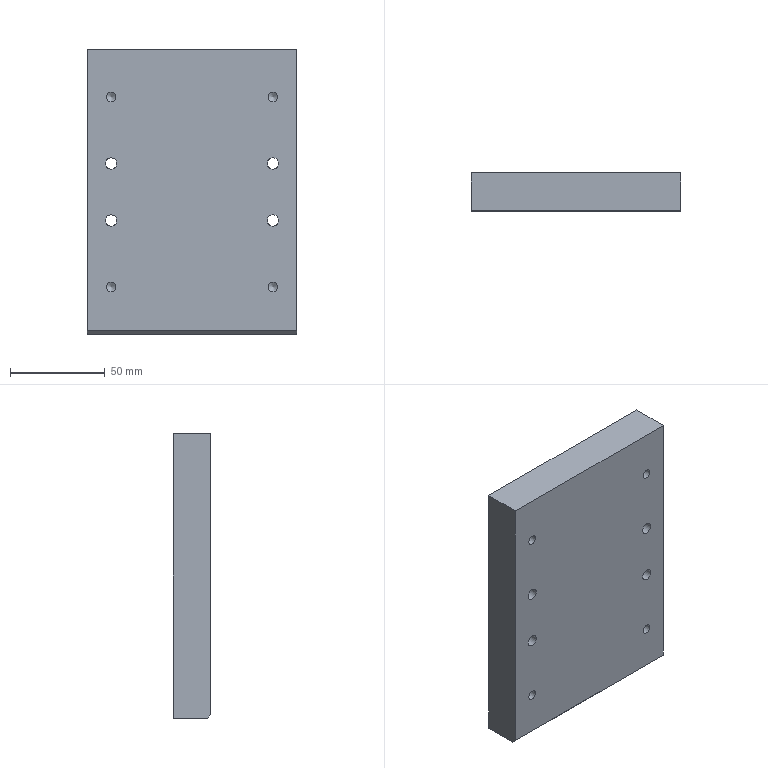Part | NX | features BREP 1 | 1 solid | 23 faces | box 110.2 x 20 x 150 mm | volume 326712 mm3 | plane 11 | cylinder 8 | cone 4 | commonest cylinder face diameters 5 x4 6 x4
STEP:
#1=CARTESIAN_POINT('',(97.7,20.,57.));
#2=VERTEX_POINT('',#1);
#3=CARTESIAN_POINT('',(97.7,20.,60.));
#4=DIRECTION('',(0.,1.,0.));
#5=DIRECTION('',(0.,0.,-1.));
#6=AXIS2_PLACEMENT_3D('',#3,#4,#5);
#7=CIRCLE('',#6,3.);
#8=EDGE_CURVE('',#2,#2,#7,.T.);
#9=ORIENTED_EDGE('',*,*,#8,.F.);
#10=EDGE_LOOP('',(#9));
#11=FACE_BOUND('',#10,.T.);
#12=CARTESIAN_POINT('',(97.7,20.,87.));
#13=VERTEX_POINT('',#12);
#14=CARTESIAN_POINT('',(97.7,20.,90.));
#15=DIRECTION('',(0.,1.,0.));
#16=DIRECTION('',(0.,0.,-1.));
#17=AXIS2_PLACEMENT_3D('',#14,#15,#16);
#18=CIRCLE('',#17,3.);
#19=EDGE_CURVE('',#13,#13,#18,.T.);
#20=ORIENTED_EDGE('',*,*,#19,.F.);
#21=EDGE_LOOP('',(#20));
#22=FACE_BOUND('',#21,.T.);
#23=CARTESIAN_POINT('',(12.5,20.,57.));
#24=VERTEX_POINT('',#23);
#25=CARTESIAN_POINT('',(12.5,20.,60.));
#26=DIRECTION('',(0.,1.,0.));
#27=DIRECTION('',(0.,0.,-1.));
#28=AXIS2_PLACEMENT_3D('',#25,#26,#27);
#29=CIRCLE('',#28,3.);
#30=EDGE_CURVE('',#24,#24,#29,.T.);
#31=ORIENTED_EDGE('',*,*,#30,.F.);
#32=EDGE_LOOP('',(#31));
#33=FACE_BOUND('',#32,.T.);
#34=CARTESIAN_POINT('',(12.5,20.,87.));
#35=VERTEX_POINT('',#34);
#36=CARTESIAN_POINT('',(12.5,20.,90.));
#37=DIRECTION('',(0.,1.,0.));
#38=DIRECTION('',(0.,0.,-1.));
#39=AXIS2_PLACEMENT_3D('',#36,#37,#38);
#40=CIRCLE('',#39,3.);
#41=EDGE_CURVE('',#35,#35,#40,.T.);
#42=ORIENTED_EDGE('',*,*,#41,.F.);
#43=EDGE_LOOP('',(#42));
#44=FACE_BOUND('',#43,.T.);
#45=CARTESIAN_POINT('',(0.,20.,0.));
#46=VERTEX_POINT('',#45);
#47=CARTESIAN_POINT('',(110.2,20.,0.));
#48=VERTEX_POINT('',#47);
#49=CARTESIAN_POINT('',(0.,20.,0.));
#50=DIRECTION('',(1.,0.,0.));
#51=VECTOR('',#50,1000.);
#52=LINE('',#49,#51);
#53=EDGE_CURVE('',#46,#48,#52,.T.);
#54=ORIENTED_EDGE('',*,*,#53,.F.);
#55=CARTESIAN_POINT('',(0.,20.,150.));
#56=VERTEX_POINT('',#55);
#57=CARTESIAN_POINT('',(0.,20.,150.));
#58=DIRECTION('',(0.,0.,-1.));
#59=VECTOR('',#58,1000.);
#60=LINE('',#57,#59);
#61=EDGE_CURVE('',#56,#46,#60,.T.);
#62=ORIENTED_EDGE('',*,*,#61,.F.);
#63=CARTESIAN_POINT('',(110.2,20.,150.));
#64=VERTEX_POINT('',#63);
#65=CARTESIAN_POINT('',(0.,20.,150.));
#66=DIRECTION('',(1.,0.,0.));
#67=VECTOR('',#66,1000.);
#68=LINE('',#65,#67);
#69=EDGE_CURVE('',#56,#64,#68,.T.);
#70=ORIENTED_EDGE('',*,*,#69,.T.);
#71=CARTESIAN_POINT('',(110.2,20.,150.));
#72=DIRECTION('',(0.,0.,-1.));
#73=VECTOR('',#72,1000.);
#74=LINE('',#71,#73);
#75=EDGE_CURVE('',#64,#48,#74,.T.);
#76=ORIENTED_EDGE('',*,*,#75,.T.);
#77=EDGE_LOOP('',(#54,#62,#70,#76));
#78=FACE_BOUND('',#77,.T.);
#79=CARTESIAN_POINT('',(0.,20.,150.));
#80=DIRECTION('',(0.,1.,0.));
#81=DIRECTION('',(1.,0.,0.));
#82=AXIS2_PLACEMENT_3D('',#79,#80,#81);
#83=PLANE('',#82);
#84=ADVANCED_FACE('',(#11,#22,#33,#44,#78),#83,.T.);
#85=CARTESIAN_POINT('',(110.2,0.,150.));
#86=VERTEX_POINT('',#85);
#87=CARTESIAN_POINT('',(110.2,0.,2.));
#88=VERTEX_POINT('',#87);
#89=CARTESIAN_POINT('',(110.2,0.,150.));
#90=DIRECTION('',(0.,0.,-1.));
#91=VECTOR('',#90,1000.);
#92=LINE('',#89,#91);
#93=EDGE_CURVE('',#86,#88,#92,.T.);
#94=ORIENTED_EDGE('',*,*,#93,.T.);
#95=CARTESIAN_POINT('',(110.2,2.,0.));
#96=VERTEX_POINT('',#95);
#97=CARTESIAN_POINT('',(110.2,-64.,66.));
#98=DIRECTION('',(0.,0.7071,-0.7071));
#99=VECTOR('',#98,1000.);
#100=LINE('',#97,#99);
#101=EDGE_CURVE('',#88,#96,#100,.T.);
#102=ORIENTED_EDGE('',*,*,#101,.T.);
#103=CARTESIAN_POINT('',(110.2,20.,0.));
#104=DIRECTION('',(0.,-1.,0.));
#105=VECTOR('',#104,1000.);
#106=LINE('',#103,#105);
#107=EDGE_CURVE('',#48,#96,#106,.T.);
#108=ORIENTED_EDGE('',*,*,#107,.F.);
#109=ORIENTED_EDGE('',*,*,#75,.F.);
#110=CARTESIAN_POINT('',(110.2,20.,150.));
#111=DIRECTION('',(0.,-1.,0.));
#112=VECTOR('',#111,1000.);
#113=LINE('',#110,#112);
#114=EDGE_CURVE('',#64,#86,#113,.T.);
#115=ORIENTED_EDGE('',*,*,#114,.T.);
#116=EDGE_LOOP('',(#94,#102,#108,#109,#115));
#117=FACE_BOUND('',#116,.T.);
#118=CARTESIAN_POINT('',(110.2,20.,150.));
#119=DIRECTION('',(1.,0.,0.));
#120=DIRECTION('',(0.,0.,1.));
#121=AXIS2_PLACEMENT_3D('',#118,#119,#120);
#122=PLANE('',#121);
#123=ADVANCED_FACE('',(#117),#122,.T.);
#124=CARTESIAN_POINT('',(100.7,0.,60.));
#125=VERTEX_POINT('',#124);
#126=CARTESIAN_POINT('',(97.7,0.,60.));
#127=DIRECTION('',(0.,-1.,0.));
#128=DIRECTION('',(1.,0.,0.));
#129=AXIS2_PLACEMENT_3D('',#126,#127,#128);
#130=CIRCLE('',#129,3.);
#131=EDGE_CURVE('',#125,#125,#130,.T.);
#132=ORIENTED_EDGE('',*,*,#131,.F.);
#133=EDGE_LOOP('',(#132));
#134=FACE_BOUND('',#133,.T.);
#135=CARTESIAN_POINT('',(100.7,0.,90.));
#136=VERTEX_POINT('',#135);
#137=CARTESIAN_POINT('',(97.7,0.,90.));
#138=DIRECTION('',(0.,-1.,0.));
#139=DIRECTION('',(1.,0.,0.));
#140=AXIS2_PLACEMENT_3D('',#137,#138,#139);
#141=CIRCLE('',#140,3.);
#142=EDGE_CURVE('',#136,#136,#141,.T.);
#143=ORIENTED_EDGE('',*,*,#142,.F.);
#144=EDGE_LOOP('',(#143));
#145=FACE_BOUND('',#144,.T.);
#146=CARTESIAN_POINT('',(15.5,0.,60.));
#147=VERTEX_POINT('',#146);
#148=CARTESIAN_POINT('',(12.5,0.,60.));
#149=DIRECTION('',(0.,-1.,0.));
#150=DIRECTION('',(1.,0.,0.));
#151=AXIS2_PLACEMENT_3D('',#148,#149,#150);
#152=CIRCLE('',#151,3.);
#153=EDGE_CURVE('',#147,#147,#152,.T.);
#154=ORIENTED_EDGE('',*,*,#153,.F.);
#155=EDGE_LOOP('',(#154));
#156=FACE_BOUND('',#155,.T.);
#157=CARTESIAN_POINT('',(15.5,0.,90.));
#158=VERTEX_POINT('',#157);
#159=CARTESIAN_POINT('',(12.5,0.,90.));
#160=DIRECTION('',(0.,-1.,0.));
#161=DIRECTION('',(1.,0.,0.));
#162=AXIS2_PLACEMENT_3D('',#159,#160,#161);
#163=CIRCLE('',#162,3.);
#164=EDGE_CURVE('',#158,#158,#163,.T.);
#165=ORIENTED_EDGE('',*,*,#164,.F.);
#166=EDGE_LOOP('',(#165));
#167=FACE_BOUND('',#166,.T.);
#168=CARTESIAN_POINT('',(0.,0.,150.));
#169=VERTEX_POINT('',#168);
#170=CARTESIAN_POINT('',(0.,0.,2.));
#171=VERTEX_POINT('',#170);
#172=CARTESIAN_POINT('',(0.,0.,150.));
#173=DIRECTION('',(0.,0.,-1.));
#174=VECTOR('',#173,1000.);
#175=LINE('',#172,#174);
#176=EDGE_CURVE('',#169,#171,#175,.T.);
#177=ORIENTED_EDGE('',*,*,#176,.T.);
#178=CARTESIAN_POINT('',(110.2,0.,2.));
#179=DIRECTION('',(1.,0.,0.));
#180=VECTOR('',#179,1000.);
#181=LINE('',#178,#180);
#182=EDGE_CURVE('',#171,#88,#181,.T.);
#183=ORIENTED_EDGE('',*,*,#182,.T.);
#184=ORIENTED_EDGE('',*,*,#93,.F.);
#185=CARTESIAN_POINT('',(110.2,0.,150.));
#186=DIRECTION('',(-1.,0.,0.));
#187=VECTOR('',#186,1000.);
#188=LINE('',#185,#187);
#189=EDGE_CURVE('',#86,#169,#188,.T.);
#190=ORIENTED_EDGE('',*,*,#189,.T.);
#191=EDGE_LOOP('',(#177,#183,#184,#190));
#192=FACE_BOUND('',#191,.T.);
#193=CARTESIAN_POINT('',(12.5,0.,122.5));
#194=VERTEX_POINT('',#193);
#195=CARTESIAN_POINT('',(12.5,0.,125.));
#196=DIRECTION('',(0.,-1.,0.));
#197=DIRECTION('',(0.,0.,-1.));
#198=AXIS2_PLACEMENT_3D('',#195,#196,#197);
#199=CIRCLE('',#198,2.5);
#200=EDGE_CURVE('',#194,#194,#199,.T.);
#201=ORIENTED_EDGE('',*,*,#200,.F.);
#202=EDGE_LOOP('',(#201));
#203=FACE_BOUND('',#202,.T.);
#204=CARTESIAN_POINT('',(12.5,0.,22.5));
#205=VERTEX_POINT('',#204);
#206=CARTESIAN_POINT('',(12.5,0.,25.));
#207=DIRECTION('',(0.,-1.,0.));
#208=DIRECTION('',(0.,0.,-1.));
#209=AXIS2_PLACEMENT_3D('',#206,#207,#208);
#210=CIRCLE('',#209,2.5);
#211=EDGE_CURVE('',#205,#205,#210,.T.);
#212=ORIENTED_EDGE('',*,*,#211,.F.);
#213=EDGE_LOOP('',(#212));
#214=FACE_BOUND('',#213,.T.);
#215=CARTESIAN_POINT('',(97.7,0.,122.5));
#216=VERTEX_POINT('',#215);
#217=CARTESIAN_POINT('',(97.7,0.,125.));
#218=DIRECTION('',(0.,-1.,0.));
#219=DIRECTION('',(0.,0.,-1.));
#220=AXIS2_PLACEMENT_3D('',#217,#218,#219);
#221=CIRCLE('',#220,2.5);
#222=EDGE_CURVE('',#216,#216,#221,.T.);
#223=ORIENTED_EDGE('',*,*,#222,.F.);
#224=EDGE_LOOP('',(#223));
#225=FACE_BOUND('',#224,.T.);
#226=CARTESIAN_POINT('',(97.7,0.,22.5));
#227=VERTEX_POINT('',#226);
#228=CARTESIAN_POINT('',(97.7,0.,25.));
#229=DIRECTION('',(0.,-1.,0.));
#230=DIRECTION('',(0.,0.,-1.));
#231=AXIS2_PLACEMENT_3D('',#228,#229,#230);
#232=CIRCLE('',#231,2.5);
#233=EDGE_CURVE('',#227,#227,#232,.T.);
#234=ORIENTED_EDGE('',*,*,#233,.F.);
#235=EDGE_LOOP('',(#234));
#236=FACE_BOUND('',#235,.T.);
#237=CARTESIAN_POINT('',(110.2,0.,150.));
#238=DIRECTION('',(0.,-1.,0.));
#239=DIRECTION('',(-1.,0.,0.));
#240=AXIS2_PLACEMENT_3D('',#237,#238,#239);
#241=PLANE('',#240);
#242=ADVANCED_FACE('',(#134,#145,#156,#167,#192,#203,#214,#225,#236),#241,.T.);
#243=CARTESIAN_POINT('',(0.,2.,0.));
#244=VERTEX_POINT('',#243);
#245=CARTESIAN_POINT('',(0.,0.,0.));
#246=DIRECTION('',(0.,1.,0.));
#247=VECTOR('',#246,1000.);
#248=LINE('',#245,#247);
#249=EDGE_CURVE('',#244,#46,#248,.T.);
#250=ORIENTED_EDGE('',*,*,#249,.F.);
#251=CARTESIAN_POINT('',(0.,-74.,76.));
#252=DIRECTION('',(0.,-0.7071,0.7071));
#253=VECTOR('',#252,1000.);
#254=LINE('',#251,#253);
#255=EDGE_CURVE('',#244,#171,#254,.T.);
#256=ORIENTED_EDGE('',*,*,#255,.T.);
#257=ORIENTED_EDGE('',*,*,#176,.F.);
#258=CARTESIAN_POINT('',(0.,0.,150.));
#259=DIRECTION('',(0.,1.,0.));
#260=VECTOR('',#259,1000.);
#261=LINE('',#258,#260);
#262=EDGE_CURVE('',#169,#56,#261,.T.);
#263=ORIENTED_EDGE('',*,*,#262,.T.);
#264=ORIENTED_EDGE('',*,*,#61,.T.);
#265=EDGE_LOOP('',(#250,#256,#257,#263,#264));
#266=FACE_BOUND('',#265,.T.);
#267=CARTESIAN_POINT('',(0.,0.,150.));
#268=DIRECTION('',(-1.,0.,0.));
#269=DIRECTION('',(0.,1.,0.));
#270=AXIS2_PLACEMENT_3D('',#267,#268,#269);
#271=PLANE('',#270);
#272=ADVANCED_FACE('',(#266),#271,.T.);
#273=ORIENTED_EDGE('',*,*,#69,.F.);
#274=ORIENTED_EDGE('',*,*,#262,.F.);
#275=ORIENTED_EDGE('',*,*,#189,.F.);
#276=ORIENTED_EDGE('',*,*,#114,.F.);
#277=EDGE_LOOP('',(#273,#274,#275,#276));
#278=FACE_BOUND('',#277,.T.);
#279=CARTESIAN_POINT('',(110.2,20.,150.));
#280=DIRECTION('',(0.,0.,-1.));
#281=DIRECTION('',(1.,0.,0.));
#282=AXIS2_PLACEMENT_3D('',#279,#280,#281);
#283=PLANE('',#282);
#284=ADVANCED_FACE('',(#278),#283,.F.);
#285=ORIENTED_EDGE('',*,*,#107,.T.);
#286=CARTESIAN_POINT('',(110.2,2.,0.));
#287=DIRECTION('',(-1.,0.,0.));
#288=VECTOR('',#287,1000.);
#289=LINE('',#286,#288);
#290=EDGE_CURVE('',#96,#244,#289,.T.);
#291=ORIENTED_EDGE('',*,*,#290,.T.);
#292=ORIENTED_EDGE('',*,*,#249,.T.);
#293=ORIENTED_EDGE('',*,*,#53,.T.);
#294=EDGE_LOOP('',(#285,#291,#292,#293));
#295=FACE_BOUND('',#294,.T.);
#296=CARTESIAN_POINT('',(110.2,20.,0.));
#297=DIRECTION('',(0.,0.,-1.));
#298=DIRECTION('',(1.,0.,0.));
#299=AXIS2_PLACEMENT_3D('',#296,#297,#298);
#300=PLANE('',#299);
#301=ADVANCED_FACE('',(#295),#300,.T.);
#302=ORIENTED_EDGE('',*,*,#101,.F.);
#303=ORIENTED_EDGE('',*,*,#182,.F.);
#304=ORIENTED_EDGE('',*,*,#255,.F.);
#305=ORIENTED_EDGE('',*,*,#290,.F.);
#306=EDGE_LOOP('',(#302,#303,#304,#305));
#307=FACE_BOUND('',#306,.T.);
#308=CARTESIAN_POINT('',(110.2,2.,0.));
#309=DIRECTION('',(0.,0.7071,0.7071));
#310=DIRECTION('',(0.,0.7071,-0.7071));
#311=AXIS2_PLACEMENT_3D('',#308,#309,#310);
#312=PLANE('',#311);
#313=ADVANCED_FACE('',(#307),#312,.F.);
#314=ORIENTED_EDGE('',*,*,#200,.T.);
#315=EDGE_LOOP('',(#314));
#316=FACE_BOUND('',#315,.T.);
#317=CARTESIAN_POINT('',(12.5,17.4,122.5));
#318=VERTEX_POINT('',#317);
#319=CARTESIAN_POINT('',(12.5,17.4,125.));
#320=DIRECTION('',(0.,-1.,0.));
#321=DIRECTION('',(0.,0.,-1.));
#322=AXIS2_PLACEMENT_3D('',#319,#320,#321);
#323=CIRCLE('',#322,2.5);
#324=EDGE_CURVE('',#318,#318,#323,.T.);
#325=ORIENTED_EDGE('',*,*,#324,.F.);
#326=EDGE_LOOP('',(#325));
#327=FACE_BOUND('',#326,.T.);
#328=CARTESIAN_POINT('',(12.5,17.4,125.));
#329=DIRECTION('',(0.,-1.,0.));
#330=DIRECTION('',(0.,0.,-1.));
#331=AXIS2_PLACEMENT_3D('',#328,#329,#330);
#332=CYLINDRICAL_SURFACE('',#331,2.5);
#333=ADVANCED_FACE('',(#316,#327),#332,.F.);
#334=CARTESIAN_POINT('',(12.5,18.83,124.881));
#335=VERTEX_POINT('',#334);
#336=CARTESIAN_POINT('',(12.5,18.83,125.));
#337=DIRECTION('',(0.,-1.,0.));
#338=DIRECTION('',(0.,0.,-1.));
#339=AXIS2_PLACEMENT_3D('',#336,#337,#338);
#340=CIRCLE('',#339,0.1193);
#341=EDGE_CURVE('',#335,#335,#340,.T.);
#342=ORIENTED_EDGE('',*,*,#341,.T.);
#343=EDGE_LOOP('',(#342));
#344=FACE_BOUND('',#343,.T.);
#345=CARTESIAN_POINT('',(12.5,18.83,125.));
#346=DIRECTION('',(0.,1.,0.));
#347=DIRECTION('',(0.,0.,1.));
#348=AXIS2_PLACEMENT_3D('',#345,#346,#347);
#349=PLANE('',#348);
#350=ADVANCED_FACE('',(#344),#349,.F.);
#351=ORIENTED_EDGE('',*,*,#341,.F.);
#352=EDGE_LOOP('',(#351));
#353=FACE_BOUND('',#352,.T.);
#354=ORIENTED_EDGE('',*,*,#324,.T.);
#355=EDGE_LOOP('',(#354));
#356=FACE_BOUND('',#355,.T.);
#357=CARTESIAN_POINT('',(12.5,17.4,125.));
#358=DIRECTION('',(0.,-1.,0.));
#359=DIRECTION('',(0.,0.,-1.));
#360=AXIS2_PLACEMENT_3D('',#357,#358,#359);
#361=CONICAL_SURFACE('',#360,2.5,1.03);
#362=ADVANCED_FACE('',(#353,#356),#361,.F.);
#363=ORIENTED_EDGE('',*,*,#211,.T.);
#364=EDGE_LOOP('',(#363));
#365=FACE_BOUND('',#364,.T.);
#366=CARTESIAN_POINT('',(12.5,17.4,22.5));
#367=VERTEX_POINT('',#366);
#368=CARTESIAN_POINT('',(12.5,17.4,25.));
#369=DIRECTION('',(0.,-1.,0.));
#370=DIRECTION('',(0.,0.,-1.));
#371=AXIS2_PLACEMENT_3D('',#368,#369,#370);
#372=CIRCLE('',#371,2.5);
#373=EDGE_CURVE('',#367,#367,#372,.T.);
#374=ORIENTED_EDGE('',*,*,#373,.F.);
#375=EDGE_LOOP('',(#374));
#376=FACE_BOUND('',#375,.T.);
#377=CARTESIAN_POINT('',(12.5,17.4,25.));
#378=DIRECTION('',(0.,-1.,0.));
#379=DIRECTION('',(0.,0.,-1.));
#380=AXIS2_PLACEMENT_3D('',#377,#378,#379);
#381=CYLINDRICAL_SURFACE('',#380,2.5);
#382=ADVANCED_FACE('',(#365,#376),#381,.F.);
#383=CARTESIAN_POINT('',(12.5,18.83,24.881));
#384=VERTEX_POINT('',#383);
#385=CARTESIAN_POINT('',(12.5,18.83,25.));
#386=DIRECTION('',(0.,-1.,0.));
#387=DIRECTION('',(0.,0.,-1.));
#388=AXIS2_PLACEMENT_3D('',#385,#386,#387);
#389=CIRCLE('',#388,0.1193);
#390=EDGE_CURVE('',#384,#384,#389,.T.);
#391=ORIENTED_EDGE('',*,*,#390,.T.);
#392=EDGE_LOOP('',(#391));
#393=FACE_BOUND('',#392,.T.);
#394=CARTESIAN_POINT('',(12.5,18.83,25.));
#395=DIRECTION('',(0.,1.,0.));
#396=DIRECTION('',(0.,0.,1.));
#397=AXIS2_PLACEMENT_3D('',#394,#395,#396);
#398=PLANE('',#397);
#399=ADVANCED_FACE('',(#393),#398,.F.);
#400=ORIENTED_EDGE('',*,*,#390,.F.);
#401=EDGE_LOOP('',(#400));
#402=FACE_BOUND('',#401,.T.);
#403=ORIENTED_EDGE('',*,*,#373,.T.);
#404=EDGE_LOOP('',(#403));
#405=FACE_BOUND('',#404,.T.);
#406=CARTESIAN_POINT('',(12.5,17.4,25.));
#407=DIRECTION('',(0.,-1.,0.));
#408=DIRECTION('',(0.,0.,-1.));
#409=AXIS2_PLACEMENT_3D('',#406,#407,#408);
#410=CONICAL_SURFACE('',#409,2.5,1.03);
#411=ADVANCED_FACE('',(#402,#405),#410,.F.);
#412=ORIENTED_EDGE('',*,*,#164,.T.);
#413=EDGE_LOOP('',(#412));
#414=FACE_BOUND('',#413,.T.);
#415=ORIENTED_EDGE('',*,*,#41,.T.);
#416=EDGE_LOOP('',(#415));
#417=FACE_BOUND('',#416,.T.);
#418=CARTESIAN_POINT('',(12.5,-13.1,90.));
#419=DIRECTION('',(0.,1.,0.));
#420=DIRECTION('',(0.,0.,1.));
#421=AXIS2_PLACEMENT_3D('',#418,#419,#420);
#422=CYLINDRICAL_SURFACE('',#421,3.);
#423=ADVANCED_FACE('',(#414,#417),#422,.F.);
#424=ORIENTED_EDGE('',*,*,#153,.T.);
#425=EDGE_LOOP('',(#424));
#426=FACE_BOUND('',#425,.T.);
#427=ORIENTED_EDGE('',*,*,#30,.T.);
#428=EDGE_LOOP('',(#427));
#429=FACE_BOUND('',#428,.T.);
#430=CARTESIAN_POINT('',(12.5,-13.1,60.));
#431=DIRECTION('',(0.,1.,0.));
#432=DIRECTION('',(0.,0.,1.));
#433=AXIS2_PLACEMENT_3D('',#430,#431,#432);
#434=CYLINDRICAL_SURFACE('',#433,3.);
#435=ADVANCED_FACE('',(#426,#429),#434,.F.);
#436=ORIENTED_EDGE('',*,*,#222,.T.);
#437=EDGE_LOOP('',(#436));
#438=FACE_BOUND('',#437,.T.);
#439=CARTESIAN_POINT('',(97.7,17.4,122.5));
#440=VERTEX_POINT('',#439);
#441=CARTESIAN_POINT('',(97.7,17.4,125.));
#442=DIRECTION('',(0.,-1.,0.));
#443=DIRECTION('',(0.,0.,-1.));
#444=AXIS2_PLACEMENT_3D('',#441,#442,#443);
#445=CIRCLE('',#444,2.5);
#446=EDGE_CURVE('',#440,#440,#445,.T.);
#447=ORIENTED_EDGE('',*,*,#446,.F.);
#448=EDGE_LOOP('',(#447));
#449=FACE_BOUND('',#448,.T.);
#450=CARTESIAN_POINT('',(97.7,17.4,125.));
#451=DIRECTION('',(0.,-1.,0.));
#452=DIRECTION('',(0.,0.,-1.));
#453=AXIS2_PLACEMENT_3D('',#450,#451,#452);
#454=CYLINDRICAL_SURFACE('',#453,2.5);
#455=ADVANCED_FACE('',(#438,#449),#454,.F.);
#456=CARTESIAN_POINT('',(97.7,18.83,124.881));
#457=VERTEX_POINT('',#456);
#458=CARTESIAN_POINT('',(97.7,18.83,125.));
#459=DIRECTION('',(0.,-1.,0.));
#460=DIRECTION('',(0.,0.,-1.));
#461=AXIS2_PLACEMENT_3D('',#458,#459,#460);
#462=CIRCLE('',#461,0.1193);
#463=EDGE_CURVE('',#457,#457,#462,.T.);
#464=ORIENTED_EDGE('',*,*,#463,.T.);
#465=EDGE_LOOP('',(#464));
#466=FACE_BOUND('',#465,.T.);
#467=CARTESIAN_POINT('',(97.7,18.83,125.));
#468=DIRECTION('',(0.,1.,0.));
#469=DIRECTION('',(0.,0.,1.));
#470=AXIS2_PLACEMENT_3D('',#467,#468,#469);
#471=PLANE('',#470);
#472=ADVANCED_FACE('',(#466),#471,.F.);
#473=ORIENTED_EDGE('',*,*,#463,.F.);
#474=EDGE_LOOP('',(#473));
#475=FACE_BOUND('',#474,.T.);
#476=ORIENTED_EDGE('',*,*,#446,.T.);
#477=EDGE_LOOP('',(#476));
#478=FACE_BOUND('',#477,.T.);
#479=CARTESIAN_POINT('',(97.7,17.4,125.));
#480=DIRECTION('',(0.,-1.,0.));
#481=DIRECTION('',(0.,0.,-1.));
#482=AXIS2_PLACEMENT_3D('',#479,#480,#481);
#483=CONICAL_SURFACE('',#482,2.5,1.03);
#484=ADVANCED_FACE('',(#475,#478),#483,.F.);
#485=ORIENTED_EDGE('',*,*,#233,.T.);
#486=EDGE_LOOP('',(#485));
#487=FACE_BOUND('',#486,.T.);
#488=CARTESIAN_POINT('',(97.7,17.4,22.5));
#489=VERTEX_POINT('',#488);
#490=CARTESIAN_POINT('',(97.7,17.4,25.));
#491=DIRECTION('',(0.,-1.,0.));
#492=DIRECTION('',(0.,0.,-1.));
#493=AXIS2_PLACEMENT_3D('',#490,#491,#492);
#494=CIRCLE('',#493,2.5);
#495=EDGE_CURVE('',#489,#489,#494,.T.);
#496=ORIENTED_EDGE('',*,*,#495,.F.);
#497=EDGE_LOOP('',(#496));
#498=FACE_BOUND('',#497,.T.);
#499=CARTESIAN_POINT('',(97.7,17.4,25.));
#500=DIRECTION('',(0.,-1.,0.));
#501=DIRECTION('',(0.,0.,-1.));
#502=AXIS2_PLACEMENT_3D('',#499,#500,#501);
#503=CYLINDRICAL_SURFACE('',#502,2.5);
#504=ADVANCED_FACE('',(#487,#498),#503,.F.);
#505=CARTESIAN_POINT('',(97.7,18.83,24.881));
#506=VERTEX_POINT('',#505);
#507=CARTESIAN_POINT('',(97.7,18.83,25.));
#508=DIRECTION('',(0.,-1.,0.));
#509=DIRECTION('',(0.,0.,-1.));
#510=AXIS2_PLACEMENT_3D('',#507,#508,#509);
#511=CIRCLE('',#510,0.1193);
#512=EDGE_CURVE('',#506,#506,#511,.T.);
#513=ORIENTED_EDGE('',*,*,#512,.T.);
#514=EDGE_LOOP('',(#513));
#515=FACE_BOUND('',#514,.T.);
#516=CARTESIAN_POINT('',(97.7,18.83,25.));
#517=DIRECTION('',(0.,1.,0.));
#518=DIRECTION('',(0.,0.,1.));
#519=AXIS2_PLACEMENT_3D('',#516,#517,#518);
#520=PLANE('',#519);
#521=ADVANCED_FACE('',(#515),#520,.F.);
#522=ORIENTED_EDGE('',*,*,#512,.F.);
#523=EDGE_LOOP('',(#522));
#524=FACE_BOUND('',#523,.T.);
#525=ORIENTED_EDGE('',*,*,#495,.T.);
#526=EDGE_LOOP('',(#525));
#527=FACE_BOUND('',#526,.T.);
#528=CARTESIAN_POINT('',(97.7,17.4,25.));
#529=DIRECTION('',(0.,-1.,0.));
#530=DIRECTION('',(0.,0.,-1.));
#531=AXIS2_PLACEMENT_3D('',#528,#529,#530);
#532=CONICAL_SURFACE('',#531,2.5,1.03);
#533=ADVANCED_FACE('',(#524,#527),#532,.F.);
#534=ORIENTED_EDGE('',*,*,#142,.T.);
#535=EDGE_LOOP('',(#534));
#536=FACE_BOUND('',#535,.T.);
#537=ORIENTED_EDGE('',*,*,#19,.T.);
#538=EDGE_LOOP('',(#537));
#539=FACE_BOUND('',#538,.T.);
#540=CARTESIAN_POINT('',(97.7,-13.1,90.));
#541=DIRECTION('',(0.,1.,0.));
#542=DIRECTION('',(0.,0.,1.));
#543=AXIS2_PLACEMENT_3D('',#540,#541,#542);
#544=CYLINDRICAL_SURFACE('',#543,3.);
#545=ADVANCED_FACE('',(#536,#539),#544,.F.);
#546=ORIENTED_EDGE('',*,*,#131,.T.);
#547=EDGE_LOOP('',(#546));
#548=FACE_BOUND('',#547,.T.);
#549=ORIENTED_EDGE('',*,*,#8,.T.);
#550=EDGE_LOOP('',(#549));
#551=FACE_BOUND('',#550,.T.);
#552=CARTESIAN_POINT('',(97.7,-13.1,60.));
#553=DIRECTION('',(0.,1.,0.));
#554=DIRECTION('',(0.,0.,1.));
#555=AXIS2_PLACEMENT_3D('',#552,#553,#554);
#556=CYLINDRICAL_SURFACE('',#555,3.);
#557=ADVANCED_FACE('',(#548,#551),#556,.F.);
#558=CLOSED_SHELL('',(#84,#123,#242,#272,#284,#301,#313,#333,#350,#362,#382,#399,#411,#423,#435,#455,#472,#484,#504,#521,#533,#545,#557));
#559=MANIFOLD_SOLID_BREP('',#558);
#560=(LENGTH_UNIT()NAMED_UNIT(*)SI_UNIT(.MILLI.,.METRE.));
#561=UNCERTAINTY_MEASURE_WITH_UNIT(LENGTH_MEASURE(0.00001),#560,'','');
#562=(NAMED_UNIT(*)PLANE_ANGLE_UNIT()SI_UNIT($,.RADIAN.));
#563=(NAMED_UNIT(*)SI_UNIT($,.STERADIAN.)SOLID_ANGLE_UNIT());
#564=(GEOMETRIC_REPRESENTATION_CONTEXT(3)GLOBAL_UNCERTAINTY_ASSIGNED_CONTEXT((#561))GLOBAL_UNIT_ASSIGNED_CONTEXT((#560,#562,#563))REPRESENTATION_CONTEXT('',''));
#565=ADVANCED_BREP_SHAPE_REPRESENTATION('',(#559),#564);